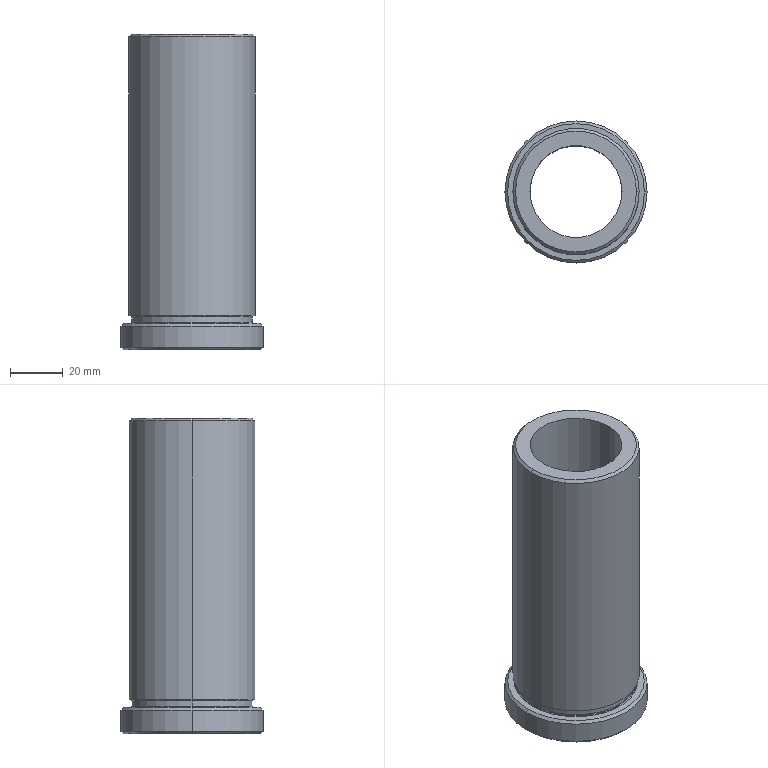Part | Creo | 1 solid | 26 faces | box 54 x 54 x 120 mm | volume 105831 mm3 | cylinder 8 | torus 8 | cone 6 | plane 4 | commonest cylinder face diameters 35 x2 46 x2 48 x2 54 x2
STEP:
#1=CARTESIAN_POINT('',(0.,0.,0.));
#2=DIRECTION('',(0.,0.,1.));
#3=DIRECTION('',(1.,0.,0.));
#4=AXIS2_PLACEMENT_3D('',#1,#2,#3);
#5=CARTESIAN_POINT('',(-189.,212.,-111.5));
#6=VERTEX_POINT('',#5);
#7=CARTESIAN_POINT('',(-135.,212.,-111.5));
#8=VERTEX_POINT('',#7);
#9=CARTESIAN_POINT('',(-162.,212.,-111.5));
#10=DIRECTION('',(0.,0.,1.));
#11=DIRECTION('',(-1.,0.,0.));
#12=AXIS2_PLACEMENT_3D('',#9,#10,#11);
#13=CIRCLE('',#12,27.);
#14=EDGE_CURVE('',#6,#8,#13,.T.);
#15=ORIENTED_EDGE('',*,*,#14,.T.);
#16=CARTESIAN_POINT('',(-135.,212.,-119.5));
#17=VERTEX_POINT('',#16);
#18=CARTESIAN_POINT('',(-135.,212.,-111.5));
#19=DIRECTION('',(0.,0.,-1.));
#20=VECTOR('',#19,8.);
#21=LINE('',#18,#20);
#22=EDGE_CURVE('',#8,#17,#21,.T.);
#23=ORIENTED_EDGE('',*,*,#22,.T.);
#24=CARTESIAN_POINT('',(-189.,212.,-119.5));
#25=VERTEX_POINT('',#24);
#26=CARTESIAN_POINT('',(-162.,212.,-119.5));
#27=DIRECTION('',(0.,0.,-1.));
#28=DIRECTION('',(1.,0.,0.));
#29=AXIS2_PLACEMENT_3D('',#26,#27,#28);
#30=CIRCLE('',#29,27.);
#31=EDGE_CURVE('',#17,#25,#30,.T.);
#32=ORIENTED_EDGE('',*,*,#31,.T.);
#33=CARTESIAN_POINT('',(-189.,212.,-111.5));
#34=DIRECTION('',(0.,0.,-1.));
#35=VECTOR('',#34,8.);
#36=LINE('',#33,#35);
#37=EDGE_CURVE('',#6,#25,#36,.T.);
#38=ORIENTED_EDGE('',*,*,#37,.F.);
#39=EDGE_LOOP('',(#15,#23,#32,#38));
#40=FACE_OUTER_BOUND('',#39,.F.);
#41=CARTESIAN_POINT('',(-162.,212.,-110.5));
#42=DIRECTION('',(0.,0.,-1.));
#43=DIRECTION('',(1.,0.,0.));
#44=AXIS2_PLACEMENT_3D('',#41,#42,#43);
#45=CYLINDRICAL_SURFACE('',#44,27.);
#46=ADVANCED_FACE('',(#40),#45,.T.);
#47=CARTESIAN_POINT('',(-188.,212.,-110.5));
#48=VERTEX_POINT('',#47);
#49=CARTESIAN_POINT('',(-136.,212.,-110.5));
#50=VERTEX_POINT('',#49);
#51=CARTESIAN_POINT('',(-162.,212.,-110.5));
#52=DIRECTION('',(0.,0.,1.));
#53=DIRECTION('',(-1.,0.,0.));
#54=AXIS2_PLACEMENT_3D('',#51,#52,#53);
#55=CIRCLE('',#54,26.);
#56=EDGE_CURVE('',#48,#50,#55,.T.);
#57=ORIENTED_EDGE('',*,*,#56,.T.);
#58=CARTESIAN_POINT('',(-136.,212.,-110.5));
#59=DIRECTION('',(0.7071,0.,-0.7071));
#60=VECTOR('',#59,1.414);
#61=LINE('',#58,#60);
#62=EDGE_CURVE('',#50,#8,#61,.T.);
#63=ORIENTED_EDGE('',*,*,#62,.T.);
#64=ORIENTED_EDGE('',*,*,#14,.F.);
#65=CARTESIAN_POINT('',(-188.,212.,-110.5));
#66=DIRECTION('',(-0.7071,0.,-0.7071));
#67=VECTOR('',#66,1.414);
#68=LINE('',#65,#67);
#69=EDGE_CURVE('',#48,#6,#68,.T.);
#70=ORIENTED_EDGE('',*,*,#69,.F.);
#71=EDGE_LOOP('',(#57,#63,#64,#70));
#72=FACE_OUTER_BOUND('',#71,.F.);
#73=CARTESIAN_POINT('',(-162.,212.,-111.));
#74=DIRECTION('',(0.,0.,-1.));
#75=DIRECTION('',(1.,0.,0.));
#76=AXIS2_PLACEMENT_3D('',#73,#74,#75);
#77=CONICAL_SURFACE('',#76,26.5,45.);
#78=ADVANCED_FACE('',(#72),#77,.T.);
#79=ORIENTED_EDGE('',*,*,#56,.F.);
#80=CARTESIAN_POINT('',(-162.,212.,-110.5));
#81=DIRECTION('',(0.,0.,1.));
#82=DIRECTION('',(1.,0.,0.));
#83=AXIS2_PLACEMENT_3D('',#80,#81,#82);
#84=CIRCLE('',#83,26.);
#85=EDGE_CURVE('',#50,#48,#84,.T.);
#86=ORIENTED_EDGE('',*,*,#85,.F.);
#87=EDGE_LOOP('',(#79,#86));
#88=FACE_OUTER_BOUND('',#87,.F.);
#89=CARTESIAN_POINT('',(-138.5,212.,-110.5));
#90=VERTEX_POINT('',#89);
#91=CARTESIAN_POINT('',(-185.5,212.,-110.5));
#92=VERTEX_POINT('',#91);
#93=CARTESIAN_POINT('',(-162.,212.,-110.5));
#94=DIRECTION('',(0.,0.,-1.));
#95=DIRECTION('',(1.,0.,0.));
#96=AXIS2_PLACEMENT_3D('',#93,#94,#95);
#97=CIRCLE('',#96,23.5);
#98=EDGE_CURVE('',#90,#92,#97,.T.);
#99=ORIENTED_EDGE('',*,*,#98,.F.);
#100=CARTESIAN_POINT('',(-162.,212.,-110.5));
#101=DIRECTION('',(0.,0.,-1.));
#102=DIRECTION('',(-1.,0.,0.));
#103=AXIS2_PLACEMENT_3D('',#100,#101,#102);
#104=CIRCLE('',#103,23.5);
#105=EDGE_CURVE('',#92,#90,#104,.T.);
#106=ORIENTED_EDGE('',*,*,#105,.F.);
#107=EDGE_LOOP('',(#99,#106));
#108=FACE_BOUND('',#107,.F.);
#109=CARTESIAN_POINT('',(-162.,212.,-110.5));
#110=DIRECTION('',(0.,0.,-1.));
#111=DIRECTION('',(1.,0.,0.));
#112=AXIS2_PLACEMENT_3D('',#109,#110,#111);
#113=PLANE('',#112);
#114=ADVANCED_FACE('',(#88,#108),#113,.F.);
#115=ORIENTED_EDGE('',*,*,#85,.T.);
#116=ORIENTED_EDGE('',*,*,#69,.T.);
#117=CARTESIAN_POINT('',(-162.,212.,-111.5));
#118=DIRECTION('',(0.,0.,1.));
#119=DIRECTION('',(1.,0.,0.));
#120=AXIS2_PLACEMENT_3D('',#117,#118,#119);
#121=CIRCLE('',#120,27.);
#122=EDGE_CURVE('',#8,#6,#121,.T.);
#123=ORIENTED_EDGE('',*,*,#122,.F.);
#124=ORIENTED_EDGE('',*,*,#62,.F.);
#125=EDGE_LOOP('',(#115,#116,#123,#124));
#126=FACE_OUTER_BOUND('',#125,.F.);
#127=CARTESIAN_POINT('',(-162.,212.,-111.));
#128=DIRECTION('',(0.,0.,-1.));
#129=DIRECTION('',(1.,0.,0.));
#130=AXIS2_PLACEMENT_3D('',#127,#128,#129);
#131=CONICAL_SURFACE('',#130,26.5,45.);
#132=ADVANCED_FACE('',(#126),#131,.T.);
#133=ORIENTED_EDGE('',*,*,#122,.T.);
#134=ORIENTED_EDGE('',*,*,#37,.T.);
#135=CARTESIAN_POINT('',(-162.,212.,-119.5));
#136=DIRECTION('',(0.,0.,-1.));
#137=DIRECTION('',(-1.,0.,0.));
#138=AXIS2_PLACEMENT_3D('',#135,#136,#137);
#139=CIRCLE('',#138,27.);
#140=EDGE_CURVE('',#25,#17,#139,.T.);
#141=ORIENTED_EDGE('',*,*,#140,.T.);
#142=ORIENTED_EDGE('',*,*,#22,.F.);
#143=EDGE_LOOP('',(#133,#134,#141,#142));
#144=FACE_OUTER_BOUND('',#143,.F.);
#145=CARTESIAN_POINT('',(-162.,212.,-110.5));
#146=DIRECTION('',(0.,0.,-1.));
#147=DIRECTION('',(1.,0.,0.));
#148=AXIS2_PLACEMENT_3D('',#145,#146,#147);
#149=CYLINDRICAL_SURFACE('',#148,27.);
#150=ADVANCED_FACE('',(#144),#149,.T.);
#151=ORIENTED_EDGE('',*,*,#140,.F.);
#152=CARTESIAN_POINT('',(-188.,212.,-120.5));
#153=VERTEX_POINT('',#152);
#154=CARTESIAN_POINT('',(-188.,212.,-120.5));
#155=DIRECTION('',(-0.7071,0.,0.7071));
#156=VECTOR('',#155,1.414);
#157=LINE('',#154,#156);
#158=EDGE_CURVE('',#153,#25,#157,.T.);
#159=ORIENTED_EDGE('',*,*,#158,.F.);
#160=CARTESIAN_POINT('',(-136.,212.,-120.5));
#161=VERTEX_POINT('',#160);
#162=CARTESIAN_POINT('',(-162.,212.,-120.5));
#163=DIRECTION('',(0.,0.,-1.));
#164=DIRECTION('',(-1.,0.,0.));
#165=AXIS2_PLACEMENT_3D('',#162,#163,#164);
#166=CIRCLE('',#165,26.);
#167=EDGE_CURVE('',#153,#161,#166,.T.);
#168=ORIENTED_EDGE('',*,*,#167,.T.);
#169=CARTESIAN_POINT('',(-136.,212.,-120.5));
#170=DIRECTION('',(0.7071,0.,0.7071));
#171=VECTOR('',#170,1.414);
#172=LINE('',#169,#171);
#173=EDGE_CURVE('',#161,#17,#172,.T.);
#174=ORIENTED_EDGE('',*,*,#173,.T.);
#175=EDGE_LOOP('',(#151,#159,#168,#174));
#176=FACE_OUTER_BOUND('',#175,.F.);
#177=CARTESIAN_POINT('',(-162.,212.,-120.));
#178=DIRECTION('',(0.,0.,1.));
#179=DIRECTION('',(-1.,0.,0.));
#180=AXIS2_PLACEMENT_3D('',#177,#178,#179);
#181=CONICAL_SURFACE('',#180,26.5,45.);
#182=ADVANCED_FACE('',(#176),#181,.T.);
#183=ORIENTED_EDGE('',*,*,#31,.F.);
#184=ORIENTED_EDGE('',*,*,#173,.F.);
#185=CARTESIAN_POINT('',(-162.,212.,-120.5));
#186=DIRECTION('',(0.,0.,-1.));
#187=DIRECTION('',(1.,0.,0.));
#188=AXIS2_PLACEMENT_3D('',#185,#186,#187);
#189=CIRCLE('',#188,26.);
#190=EDGE_CURVE('',#161,#153,#189,.T.);
#191=ORIENTED_EDGE('',*,*,#190,.T.);
#192=ORIENTED_EDGE('',*,*,#158,.T.);
#193=EDGE_LOOP('',(#183,#184,#191,#192));
#194=FACE_OUTER_BOUND('',#193,.F.);
#195=CARTESIAN_POINT('',(-162.,212.,-120.));
#196=DIRECTION('',(0.,0.,1.));
#197=DIRECTION('',(-1.,0.,0.));
#198=AXIS2_PLACEMENT_3D('',#195,#196,#197);
#199=CONICAL_SURFACE('',#198,26.5,45.);
#200=ADVANCED_FACE('',(#194),#199,.T.);
#201=ORIENTED_EDGE('',*,*,#167,.F.);
#202=ORIENTED_EDGE('',*,*,#190,.F.);
#203=EDGE_LOOP('',(#201,#202));
#204=FACE_OUTER_BOUND('',#203,.F.);
#205=CARTESIAN_POINT('',(-144.5,212.,-120.5));
#206=VERTEX_POINT('',#205);
#207=CARTESIAN_POINT('',(-179.5,212.,-120.5));
#208=VERTEX_POINT('',#207);
#209=CARTESIAN_POINT('',(-162.,212.,-120.5));
#210=DIRECTION('',(0.,0.,1.));
#211=DIRECTION('',(1.,0.,0.));
#212=AXIS2_PLACEMENT_3D('',#209,#210,#211);
#213=CIRCLE('',#212,17.5);
#214=EDGE_CURVE('',#206,#208,#213,.T.);
#215=ORIENTED_EDGE('',*,*,#214,.F.);
#216=CARTESIAN_POINT('',(-162.,212.,-120.5));
#217=DIRECTION('',(0.,0.,1.));
#218=DIRECTION('',(-1.,0.,0.));
#219=AXIS2_PLACEMENT_3D('',#216,#217,#218);
#220=CIRCLE('',#219,17.5);
#221=EDGE_CURVE('',#208,#206,#220,.T.);
#222=ORIENTED_EDGE('',*,*,#221,.F.);
#223=EDGE_LOOP('',(#215,#222));
#224=FACE_BOUND('',#223,.F.);
#225=CARTESIAN_POINT('',(-162.,212.,-120.5));
#226=DIRECTION('',(0.,0.,-1.));
#227=DIRECTION('',(1.,0.,0.));
#228=AXIS2_PLACEMENT_3D('',#225,#226,#227);
#229=PLANE('',#228);
#230=ADVANCED_FACE('',(#204,#224),#229,.T.);
#231=CARTESIAN_POINT('',(-179.5,212.,-0.5));
#232=VERTEX_POINT('',#231);
#233=CARTESIAN_POINT('',(-144.5,212.,-0.5));
#234=VERTEX_POINT('',#233);
#235=CARTESIAN_POINT('',(-162.,212.,-0.5));
#236=DIRECTION('',(0.,0.,-1.));
#237=DIRECTION('',(-1.,0.,0.));
#238=AXIS2_PLACEMENT_3D('',#235,#236,#237);
#239=CIRCLE('',#238,17.5);
#240=EDGE_CURVE('',#232,#234,#239,.T.);
#241=ORIENTED_EDGE('',*,*,#240,.T.);
#242=CARTESIAN_POINT('',(-144.5,212.,-120.5));
#243=DIRECTION('',(0.,0.,1.));
#244=VECTOR('',#243,120.);
#245=LINE('',#242,#244);
#246=EDGE_CURVE('',#206,#234,#245,.T.);
#247=ORIENTED_EDGE('',*,*,#246,.F.);
#248=ORIENTED_EDGE('',*,*,#214,.T.);
#249=CARTESIAN_POINT('',(-179.5,212.,-120.5));
#250=DIRECTION('',(0.,0.,1.));
#251=VECTOR('',#250,120.);
#252=LINE('',#249,#251);
#253=EDGE_CURVE('',#208,#232,#252,.T.);
#254=ORIENTED_EDGE('',*,*,#253,.T.);
#255=EDGE_LOOP('',(#241,#247,#248,#254));
#256=FACE_OUTER_BOUND('',#255,.F.);
#257=CARTESIAN_POINT('',(-162.,212.,-120.5));
#258=DIRECTION('',(0.,0.,1.));
#259=DIRECTION('',(-1.,0.,0.));
#260=AXIS2_PLACEMENT_3D('',#257,#258,#259);
#261=CYLINDRICAL_SURFACE('',#260,17.5);
#262=ADVANCED_FACE('',(#256),#261,.F.);
#263=CARTESIAN_POINT('',(-139.,212.,-0.5));
#264=VERTEX_POINT('',#263);
#265=CARTESIAN_POINT('',(-185.,212.,-0.5));
#266=VERTEX_POINT('',#265);
#267=CARTESIAN_POINT('',(-162.,212.,-0.5));
#268=DIRECTION('',(0.,0.,1.));
#269=DIRECTION('',(1.,0.,0.));
#270=AXIS2_PLACEMENT_3D('',#267,#268,#269);
#271=CIRCLE('',#270,23.);
#272=EDGE_CURVE('',#264,#266,#271,.T.);
#273=ORIENTED_EDGE('',*,*,#272,.F.);
#274=CARTESIAN_POINT('',(-162.,212.,-0.5));
#275=DIRECTION('',(0.,0.,1.));
#276=DIRECTION('',(-1.,0.,0.));
#277=AXIS2_PLACEMENT_3D('',#274,#275,#276);
#278=CIRCLE('',#277,23.);
#279=EDGE_CURVE('',#266,#264,#278,.T.);
#280=ORIENTED_EDGE('',*,*,#279,.F.);
#281=EDGE_LOOP('',(#273,#280));
#282=FACE_OUTER_BOUND('',#281,.F.);
#283=CARTESIAN_POINT('',(-162.,212.,-0.5));
#284=DIRECTION('',(0.,0.,-1.));
#285=DIRECTION('',(1.,0.,0.));
#286=AXIS2_PLACEMENT_3D('',#283,#284,#285);
#287=CIRCLE('',#286,17.5);
#288=EDGE_CURVE('',#234,#232,#287,.T.);
#289=ORIENTED_EDGE('',*,*,#288,.F.);
#290=ORIENTED_EDGE('',*,*,#240,.F.);
#291=EDGE_LOOP('',(#289,#290));
#292=FACE_BOUND('',#291,.F.);
#293=CARTESIAN_POINT('',(-162.,212.,-0.5));
#294=DIRECTION('',(0.,0.,1.));
#295=DIRECTION('',(-1.,0.,0.));
#296=AXIS2_PLACEMENT_3D('',#293,#294,#295);
#297=PLANE('',#296);
#298=ADVANCED_FACE('',(#282,#292),#297,.T.);
#299=ORIENTED_EDGE('',*,*,#288,.T.);
#300=ORIENTED_EDGE('',*,*,#253,.F.);
#301=ORIENTED_EDGE('',*,*,#221,.T.);
#302=ORIENTED_EDGE('',*,*,#246,.T.);
#303=EDGE_LOOP('',(#299,#300,#301,#302));
#304=FACE_OUTER_BOUND('',#303,.F.);
#305=CARTESIAN_POINT('',(-162.,212.,-120.5));
#306=DIRECTION('',(0.,0.,1.));
#307=DIRECTION('',(-1.,0.,0.));
#308=AXIS2_PLACEMENT_3D('',#305,#306,#307);
#309=CYLINDRICAL_SURFACE('',#308,17.5);
#310=ADVANCED_FACE('',(#304),#309,.F.);
#311=CARTESIAN_POINT('',(-138.,212.,-1.5));
#312=VERTEX_POINT('',#311);
#313=CARTESIAN_POINT('',(-186.,212.,-1.5));
#314=VERTEX_POINT('',#313);
#315=CARTESIAN_POINT('',(-162.,212.,-1.5));
#316=DIRECTION('',(0.,0.,1.));
#317=DIRECTION('',(1.,0.,0.));
#318=AXIS2_PLACEMENT_3D('',#315,#316,#317);
#319=CIRCLE('',#318,24.);
#320=EDGE_CURVE('',#312,#314,#319,.T.);
#321=ORIENTED_EDGE('',*,*,#320,.F.);
#322=CARTESIAN_POINT('',(-139.,212.,-0.5));
#323=DIRECTION('',(0.7071,0.,-0.7071));
#324=VECTOR('',#323,1.414);
#325=LINE('',#322,#324);
#326=EDGE_CURVE('',#264,#312,#325,.T.);
#327=ORIENTED_EDGE('',*,*,#326,.F.);
#328=ORIENTED_EDGE('',*,*,#272,.T.);
#329=CARTESIAN_POINT('',(-185.,212.,-0.5));
#330=DIRECTION('',(-0.7071,0.,-0.7071));
#331=VECTOR('',#330,1.414);
#332=LINE('',#329,#331);
#333=EDGE_CURVE('',#266,#314,#332,.T.);
#334=ORIENTED_EDGE('',*,*,#333,.T.);
#335=EDGE_LOOP('',(#321,#327,#328,#334));
#336=FACE_OUTER_BOUND('',#335,.F.);
#337=CARTESIAN_POINT('',(-162.,212.,-1.));
#338=DIRECTION('',(0.,0.,-1.));
#339=DIRECTION('',(1.,0.,0.));
#340=AXIS2_PLACEMENT_3D('',#337,#338,#339);
#341=CONICAL_SURFACE('',#340,23.5,45.);
#342=ADVANCED_FACE('',(#336),#341,.T.);
#343=CARTESIAN_POINT('',(-186.,212.,-107.5));
#344=VERTEX_POINT('',#343);
#345=CARTESIAN_POINT('',(-138.,212.,-107.5));
#346=VERTEX_POINT('',#345);
#347=CARTESIAN_POINT('',(-162.,212.,-107.5));
#348=DIRECTION('',(0.,0.,-1.));
#349=DIRECTION('',(-1.,0.,0.));
#350=AXIS2_PLACEMENT_3D('',#347,#348,#349);
#351=CIRCLE('',#350,24.);
#352=EDGE_CURVE('',#344,#346,#351,.T.);
#353=ORIENTED_EDGE('',*,*,#352,.T.);
#354=CARTESIAN_POINT('',(-138.,212.,-107.5));
#355=DIRECTION('',(0.,0.,1.));
#356=VECTOR('',#355,106.);
#357=LINE('',#354,#356);
#358=EDGE_CURVE('',#346,#312,#357,.T.);
#359=ORIENTED_EDGE('',*,*,#358,.T.);
#360=ORIENTED_EDGE('',*,*,#320,.T.);
#361=CARTESIAN_POINT('',(-186.,212.,-107.5));
#362=DIRECTION('',(0.,0.,1.));
#363=VECTOR('',#362,106.);
#364=LINE('',#361,#363);
#365=EDGE_CURVE('',#344,#314,#364,.T.);
#366=ORIENTED_EDGE('',*,*,#365,.F.);
#367=EDGE_LOOP('',(#353,#359,#360,#366));
#368=FACE_OUTER_BOUND('',#367,.F.);
#369=CARTESIAN_POINT('',(-162.,212.,-110.5));
#370=DIRECTION('',(0.,0.,1.));
#371=DIRECTION('',(-1.,0.,0.));
#372=AXIS2_PLACEMENT_3D('',#369,#370,#371);
#373=CYLINDRICAL_SURFACE('',#372,24.);
#374=ADVANCED_FACE('',(#368),#373,.T.);
#375=CARTESIAN_POINT('',(-162.,212.,-107.5));
#376=DIRECTION('',(0.,0.,-1.));
#377=DIRECTION('',(1.,0.,0.));
#378=AXIS2_PLACEMENT_3D('',#375,#376,#377);
#379=CIRCLE('',#378,24.);
#380=EDGE_CURVE('',#346,#344,#379,.T.);
#381=ORIENTED_EDGE('',*,*,#380,.F.);
#382=ORIENTED_EDGE('',*,*,#352,.F.);
#383=EDGE_LOOP('',(#381,#382));
#384=FACE_OUTER_BOUND('',#383,.F.);
#385=CARTESIAN_POINT('',(-138.5,212.,-107.5));
#386=VERTEX_POINT('',#385);
#387=CARTESIAN_POINT('',(-185.5,212.,-107.5));
#388=VERTEX_POINT('',#387);
#389=CARTESIAN_POINT('',(-162.,212.,-107.5));
#390=DIRECTION('',(0.,0.,1.));
#391=DIRECTION('',(1.,0.,0.));
#392=AXIS2_PLACEMENT_3D('',#389,#390,#391);
#393=CIRCLE('',#392,23.5);
#394=EDGE_CURVE('',#386,#388,#393,.T.);
#395=ORIENTED_EDGE('',*,*,#394,.F.);
#396=CARTESIAN_POINT('',(-162.,212.,-107.5));
#397=DIRECTION('',(0.,0.,1.));
#398=DIRECTION('',(-1.,0.,0.));
#399=AXIS2_PLACEMENT_3D('',#396,#397,#398);
#400=CIRCLE('',#399,23.5);
#401=EDGE_CURVE('',#388,#386,#400,.T.);
#402=ORIENTED_EDGE('',*,*,#401,.F.);
#403=EDGE_LOOP('',(#395,#402));
#404=FACE_BOUND('',#403,.F.);
#405=CARTESIAN_POINT('',(-162.,212.,-107.5));
#406=DIRECTION('',(0.,0.,1.));
#407=DIRECTION('',(-1.,0.,0.));
#408=AXIS2_PLACEMENT_3D('',#405,#406,#407);
#409=PLANE('',#408);
#410=ADVANCED_FACE('',(#384,#404),#409,.F.);
#411=ORIENTED_EDGE('',*,*,#380,.T.);
#412=ORIENTED_EDGE('',*,*,#365,.T.);
#413=CARTESIAN_POINT('',(-162.,212.,-1.5));
#414=DIRECTION('',(0.,0.,1.));
#415=DIRECTION('',(-1.,0.,0.));
#416=AXIS2_PLACEMENT_3D('',#413,#414,#415);
#417=CIRCLE('',#416,24.);
#418=EDGE_CURVE('',#314,#312,#417,.T.);
#419=ORIENTED_EDGE('',*,*,#418,.T.);
#420=ORIENTED_EDGE('',*,*,#358,.F.);
#421=EDGE_LOOP('',(#411,#412,#419,#420));
#422=FACE_OUTER_BOUND('',#421,.F.);
#423=CARTESIAN_POINT('',(-162.,212.,-110.5));
#424=DIRECTION('',(0.,0.,1.));
#425=DIRECTION('',(-1.,0.,0.));
#426=AXIS2_PLACEMENT_3D('',#423,#424,#425);
#427=CYLINDRICAL_SURFACE('',#426,24.);
#428=ADVANCED_FACE('',(#422),#427,.T.);
#429=ORIENTED_EDGE('',*,*,#418,.F.);
#430=ORIENTED_EDGE('',*,*,#333,.F.);
#431=ORIENTED_EDGE('',*,*,#279,.T.);
#432=ORIENTED_EDGE('',*,*,#326,.T.);
#433=EDGE_LOOP('',(#429,#430,#431,#432));
#434=FACE_OUTER_BOUND('',#433,.F.);
#435=CARTESIAN_POINT('',(-162.,212.,-1.));
#436=DIRECTION('',(0.,0.,-1.));
#437=DIRECTION('',(1.,0.,0.));
#438=AXIS2_PLACEMENT_3D('',#435,#436,#437);
#439=CONICAL_SURFACE('',#438,23.5,45.);
#440=ADVANCED_FACE('',(#434),#439,.T.);
#441=ORIENTED_EDGE('',*,*,#394,.T.);
#442=CARTESIAN_POINT('',(-185.146,212.,-107.646));
#443=VERTEX_POINT('',#442);
#444=CARTESIAN_POINT('',(-185.5,212.,-108.));
#445=DIRECTION('',(0.,1.,0.));
#446=DIRECTION('',(0.,0.,1.));
#447=AXIS2_PLACEMENT_3D('',#444,#445,#446);
#448=CIRCLE('',#447,0.5);
#449=EDGE_CURVE('',#388,#443,#448,.T.);
#450=ORIENTED_EDGE('',*,*,#449,.T.);
#451=CARTESIAN_POINT('',(-138.854,212.,-107.646));
#452=VERTEX_POINT('',#451);
#453=CARTESIAN_POINT('',(-162.,212.,-107.646));
#454=DIRECTION('',(0.,0.,1.));
#455=DIRECTION('',(1.,0.,0.));
#456=AXIS2_PLACEMENT_3D('',#453,#454,#455);
#457=CIRCLE('',#456,23.146);
#458=EDGE_CURVE('',#452,#443,#457,.T.);
#459=ORIENTED_EDGE('',*,*,#458,.F.);
#460=CARTESIAN_POINT('',(-138.5,212.,-108.));
#461=DIRECTION('',(0.,-1.,0.));
#462=DIRECTION('',(0.,0.,1.));
#463=AXIS2_PLACEMENT_3D('',#460,#461,#462);
#464=CIRCLE('',#463,0.5);
#465=EDGE_CURVE('',#386,#452,#464,.T.);
#466=ORIENTED_EDGE('',*,*,#465,.F.);
#467=EDGE_LOOP('',(#441,#450,#459,#466));
#468=FACE_OUTER_BOUND('',#467,.F.);
#469=CARTESIAN_POINT('',(-162.,212.,-108.));
#470=DIRECTION('',(0.,0.,1.));
#471=DIRECTION('',(-1.,0.,0.));
#472=AXIS2_PLACEMENT_3D('',#469,#470,#471);
#473=TOROIDAL_SURFACE('',#472,23.5,0.5);
#474=ADVANCED_FACE('',(#468),#473,.F.);
#475=ORIENTED_EDGE('',*,*,#401,.T.);
#476=ORIENTED_EDGE('',*,*,#465,.T.);
#477=CARTESIAN_POINT('',(-162.,212.,-107.646));
#478=DIRECTION('',(0.,0.,1.));
#479=DIRECTION('',(-1.,0.,0.));
#480=AXIS2_PLACEMENT_3D('',#477,#478,#479);
#481=CIRCLE('',#480,23.146);
#482=EDGE_CURVE('',#443,#452,#481,.T.);
#483=ORIENTED_EDGE('',*,*,#482,.F.);
#484=ORIENTED_EDGE('',*,*,#449,.F.);
#485=EDGE_LOOP('',(#475,#476,#483,#484));
#486=FACE_OUTER_BOUND('',#485,.F.);
#487=CARTESIAN_POINT('',(-162.,212.,-108.));
#488=DIRECTION('',(0.,0.,1.));
#489=DIRECTION('',(-1.,0.,0.));
#490=AXIS2_PLACEMENT_3D('',#487,#488,#489);
#491=TOROIDAL_SURFACE('',#490,23.5,0.5);
#492=ADVANCED_FACE('',(#486),#491,.F.);
#493=CARTESIAN_POINT('',(-185.,212.,-108.));
#494=VERTEX_POINT('',#493);
#495=CARTESIAN_POINT('',(-139.,212.,-108.));
#496=VERTEX_POINT('',#495);
#497=CARTESIAN_POINT('',(-162.,212.,-108.));
#498=DIRECTION('',(0.,0.,1.));
#499=DIRECTION('',(-1.,0.,0.));
#500=AXIS2_PLACEMENT_3D('',#497,#498,#499);
#501=CIRCLE('',#500,23.);
#502=EDGE_CURVE('',#494,#496,#501,.T.);
#503=ORIENTED_EDGE('',*,*,#502,.F.);
#504=CARTESIAN_POINT('',(-185.5,212.,-108.));
#505=DIRECTION('',(0.,1.,0.));
#506=DIRECTION('',(0.7071,0.,0.7071));
#507=AXIS2_PLACEMENT_3D('',#504,#505,#506);
#508=CIRCLE('',#507,0.5);
#509=EDGE_CURVE('',#443,#494,#508,.T.);
#510=ORIENTED_EDGE('',*,*,#509,.F.);
#511=ORIENTED_EDGE('',*,*,#482,.T.);
#512=CARTESIAN_POINT('',(-138.5,212.,-108.));
#513=DIRECTION('',(0.,-1.,0.));
#514=DIRECTION('',(-0.7071,0.,0.7071));
#515=AXIS2_PLACEMENT_3D('',#512,#513,#514);
#516=CIRCLE('',#515,0.5);
#517=EDGE_CURVE('',#452,#496,#516,.T.);
#518=ORIENTED_EDGE('',*,*,#517,.T.);
#519=EDGE_LOOP('',(#503,#510,#511,#518));
#520=FACE_OUTER_BOUND('',#519,.F.);
#521=CARTESIAN_POINT('',(-162.,212.,-108.));
#522=DIRECTION('',(0.,0.,1.));
#523=DIRECTION('',(-1.,0.,0.));
#524=AXIS2_PLACEMENT_3D('',#521,#522,#523);
#525=TOROIDAL_SURFACE('',#524,23.5,0.5);
#526=ADVANCED_FACE('',(#520),#525,.F.);
#527=ORIENTED_EDGE('',*,*,#502,.T.);
#528=CARTESIAN_POINT('',(-139.,212.,-110.));
#529=VERTEX_POINT('',#528);
#530=CARTESIAN_POINT('',(-139.,212.,-110.));
#531=DIRECTION('',(0.,0.,1.));
#532=VECTOR('',#531,2.);
#533=LINE('',#530,#532);
#534=EDGE_CURVE('',#529,#496,#533,.T.);
#535=ORIENTED_EDGE('',*,*,#534,.F.);
#536=CARTESIAN_POINT('',(-185.,212.,-110.));
#537=VERTEX_POINT('',#536);
#538=CARTESIAN_POINT('',(-162.,212.,-110.));
#539=DIRECTION('',(0.,0.,-1.));
#540=DIRECTION('',(1.,0.,0.));
#541=AXIS2_PLACEMENT_3D('',#538,#539,#540);
#542=CIRCLE('',#541,23.);
#543=EDGE_CURVE('',#529,#537,#542,.T.);
#544=ORIENTED_EDGE('',*,*,#543,.T.);
#545=CARTESIAN_POINT('',(-185.,212.,-110.));
#546=DIRECTION('',(0.,0.,1.));
#547=VECTOR('',#546,2.);
#548=LINE('',#545,#547);
#549=EDGE_CURVE('',#537,#494,#548,.T.);
#550=ORIENTED_EDGE('',*,*,#549,.T.);
#551=EDGE_LOOP('',(#527,#535,#544,#550));
#552=FACE_OUTER_BOUND('',#551,.F.);
#553=CARTESIAN_POINT('',(-162.,212.,-109.));
#554=DIRECTION('',(0.,0.,1.));
#555=DIRECTION('',(-1.,0.,0.));
#556=AXIS2_PLACEMENT_3D('',#553,#554,#555);
#557=CYLINDRICAL_SURFACE('',#556,23.);
#558=ADVANCED_FACE('',(#552),#557,.T.);
#559=CARTESIAN_POINT('',(-162.,212.,-108.));
#560=DIRECTION('',(0.,0.,1.));
#561=DIRECTION('',(1.,0.,0.));
#562=AXIS2_PLACEMENT_3D('',#559,#560,#561);
#563=CIRCLE('',#562,23.);
#564=EDGE_CURVE('',#496,#494,#563,.T.);
#565=ORIENTED_EDGE('',*,*,#564,.T.);
#566=ORIENTED_EDGE('',*,*,#549,.F.);
#567=CARTESIAN_POINT('',(-162.,212.,-110.));
#568=DIRECTION('',(0.,0.,-1.));
#569=DIRECTION('',(-1.,0.,0.));
#570=AXIS2_PLACEMENT_3D('',#567,#568,#569);
#571=CIRCLE('',#570,23.);
#572=EDGE_CURVE('',#537,#529,#571,.T.);
#573=ORIENTED_EDGE('',*,*,#572,.T.);
#574=ORIENTED_EDGE('',*,*,#534,.T.);
#575=EDGE_LOOP('',(#565,#566,#573,#574));
#576=FACE_OUTER_BOUND('',#575,.F.);
#577=CARTESIAN_POINT('',(-162.,212.,-109.));
#578=DIRECTION('',(0.,0.,1.));
#579=DIRECTION('',(-1.,0.,0.));
#580=AXIS2_PLACEMENT_3D('',#577,#578,#579);
#581=CYLINDRICAL_SURFACE('',#580,23.);
#582=ADVANCED_FACE('',(#576),#581,.T.);
#583=ORIENTED_EDGE('',*,*,#564,.F.);
#584=ORIENTED_EDGE('',*,*,#517,.F.);
#585=ORIENTED_EDGE('',*,*,#458,.T.);
#586=ORIENTED_EDGE('',*,*,#509,.T.);
#587=EDGE_LOOP('',(#583,#584,#585,#586));
#588=FACE_OUTER_BOUND('',#587,.F.);
#589=CARTESIAN_POINT('',(-162.,212.,-108.));
#590=DIRECTION('',(0.,0.,1.));
#591=DIRECTION('',(-1.,0.,0.));
#592=AXIS2_PLACEMENT_3D('',#589,#590,#591);
#593=TOROIDAL_SURFACE('',#592,23.5,0.5);
#594=ADVANCED_FACE('',(#588),#593,.F.);
#595=ORIENTED_EDGE('',*,*,#572,.F.);
#596=CARTESIAN_POINT('',(-185.146,212.,-110.354));
#597=VERTEX_POINT('',#596);
#598=CARTESIAN_POINT('',(-185.5,212.,-110.));
#599=DIRECTION('',(0.,1.,0.));
#600=DIRECTION('',(1.,0.,0.));
#601=AXIS2_PLACEMENT_3D('',#598,#599,#600);
#602=CIRCLE('',#601,0.5);
#603=EDGE_CURVE('',#537,#597,#602,.T.);
#604=ORIENTED_EDGE('',*,*,#603,.T.);
#605=CARTESIAN_POINT('',(-138.854,212.,-110.354));
#606=VERTEX_POINT('',#605);
#607=CARTESIAN_POINT('',(-162.,212.,-110.354));
#608=DIRECTION('',(0.,0.,1.));
#609=DIRECTION('',(1.,0.,0.));
#610=AXIS2_PLACEMENT_3D('',#607,#608,#609);
#611=CIRCLE('',#610,23.146);
#612=EDGE_CURVE('',#606,#597,#611,.T.);
#613=ORIENTED_EDGE('',*,*,#612,.F.);
#614=CARTESIAN_POINT('',(-138.5,212.,-110.));
#615=DIRECTION('',(0.,-1.,0.));
#616=DIRECTION('',(-1.,0.,0.));
#617=AXIS2_PLACEMENT_3D('',#614,#615,#616);
#618=CIRCLE('',#617,0.5);
#619=EDGE_CURVE('',#529,#606,#618,.T.);
#620=ORIENTED_EDGE('',*,*,#619,.F.);
#621=EDGE_LOOP('',(#595,#604,#613,#620));
#622=FACE_OUTER_BOUND('',#621,.F.);
#623=CARTESIAN_POINT('',(-162.,212.,-110.));
#624=DIRECTION('',(0.,0.,1.));
#625=DIRECTION('',(-1.,0.,0.));
#626=AXIS2_PLACEMENT_3D('',#623,#624,#625);
#627=TOROIDAL_SURFACE('',#626,23.5,0.5);
#628=ADVANCED_FACE('',(#622),#627,.F.);
#629=ORIENTED_EDGE('',*,*,#543,.F.);
#630=ORIENTED_EDGE('',*,*,#619,.T.);
#631=CARTESIAN_POINT('',(-162.,212.,-110.354));
#632=DIRECTION('',(0.,0.,1.));
#633=DIRECTION('',(-1.,0.,0.));
#634=AXIS2_PLACEMENT_3D('',#631,#632,#633);
#635=CIRCLE('',#634,23.146);
#636=EDGE_CURVE('',#597,#606,#635,.T.);
#637=ORIENTED_EDGE('',*,*,#636,.F.);
#638=ORIENTED_EDGE('',*,*,#603,.F.);
#639=EDGE_LOOP('',(#629,#630,#637,#638));
#640=FACE_OUTER_BOUND('',#639,.F.);
#641=CARTESIAN_POINT('',(-162.,212.,-110.));
#642=DIRECTION('',(0.,0.,1.));
#643=DIRECTION('',(-1.,0.,0.));
#644=AXIS2_PLACEMENT_3D('',#641,#642,#643);
#645=TOROIDAL_SURFACE('',#644,23.5,0.5);
#646=ADVANCED_FACE('',(#640),#645,.F.);
#647=ORIENTED_EDGE('',*,*,#98,.T.);
#648=CARTESIAN_POINT('',(-185.5,212.,-110.));
#649=DIRECTION('',(0.,1.,0.));
#650=DIRECTION('',(0.7071,0.,-0.7071));
#651=AXIS2_PLACEMENT_3D('',#648,#649,#650);
#652=CIRCLE('',#651,0.5);
#653=EDGE_CURVE('',#597,#92,#652,.T.);
#654=ORIENTED_EDGE('',*,*,#653,.F.);
#655=ORIENTED_EDGE('',*,*,#636,.T.);
#656=CARTESIAN_POINT('',(-138.5,212.,-110.));
#657=DIRECTION('',(0.,-1.,0.));
#658=DIRECTION('',(-0.7071,0.,-0.7071));
#659=AXIS2_PLACEMENT_3D('',#656,#657,#658);
#660=CIRCLE('',#659,0.5);
#661=EDGE_CURVE('',#606,#90,#660,.T.);
#662=ORIENTED_EDGE('',*,*,#661,.T.);
#663=EDGE_LOOP('',(#647,#654,#655,#662));
#664=FACE_OUTER_BOUND('',#663,.F.);
#665=CARTESIAN_POINT('',(-162.,212.,-110.));
#666=DIRECTION('',(0.,0.,1.));
#667=DIRECTION('',(-1.,0.,0.));
#668=AXIS2_PLACEMENT_3D('',#665,#666,#667);
#669=TOROIDAL_SURFACE('',#668,23.5,0.5);
#670=ADVANCED_FACE('',(#664),#669,.F.);
#671=ORIENTED_EDGE('',*,*,#105,.T.);
#672=ORIENTED_EDGE('',*,*,#661,.F.);
#673=ORIENTED_EDGE('',*,*,#612,.T.);
#674=ORIENTED_EDGE('',*,*,#653,.T.);
#675=EDGE_LOOP('',(#671,#672,#673,#674));
#676=FACE_OUTER_BOUND('',#675,.F.);
#677=CARTESIAN_POINT('',(-162.,212.,-110.));
#678=DIRECTION('',(0.,0.,1.));
#679=DIRECTION('',(-1.,0.,0.));
#680=AXIS2_PLACEMENT_3D('',#677,#678,#679);
#681=TOROIDAL_SURFACE('',#680,23.5,0.5);
#682=ADVANCED_FACE('',(#676),#681,.F.);
#683=CLOSED_SHELL('',(#46,#78,#114,#132,#150,#182,#200,#230,#262,#298,#310,#342,#374,#410,#428,#440,#474,#492,#526,#558,#582,#594,#628,#646,#670,#682));
#684=MANIFOLD_SOLID_BREP('',#683);
#685=(LENGTH_UNIT()NAMED_UNIT(*)SI_UNIT(.MILLI.,.METRE.));
#686=UNCERTAINTY_MEASURE_WITH_UNIT(LENGTH_MEASURE(0.01422),#685,'','');
#687=(NAMED_UNIT(*)PLANE_ANGLE_UNIT()SI_UNIT($,.RADIAN.));
#688=PLANE_ANGLE_MEASURE_WITH_UNIT(PLANE_ANGLE_MEASURE(0.01745),#687);
#689=(CONVERSION_BASED_UNIT('DEGREE',#688)NAMED_UNIT(*)PLANE_ANGLE_UNIT());
#690=(NAMED_UNIT(*)SI_UNIT($,.STERADIAN.)SOLID_ANGLE_UNIT());
#691=(GEOMETRIC_REPRESENTATION_CONTEXT(3)GLOBAL_UNCERTAINTY_ASSIGNED_CONTEXT((#686))GLOBAL_UNIT_ASSIGNED_CONTEXT((#685,#689,#690))REPRESENTATION_CONTEXT('',''));
#692=ADVANCED_BREP_SHAPE_REPRESENTATION('',(#4,#684),#691);